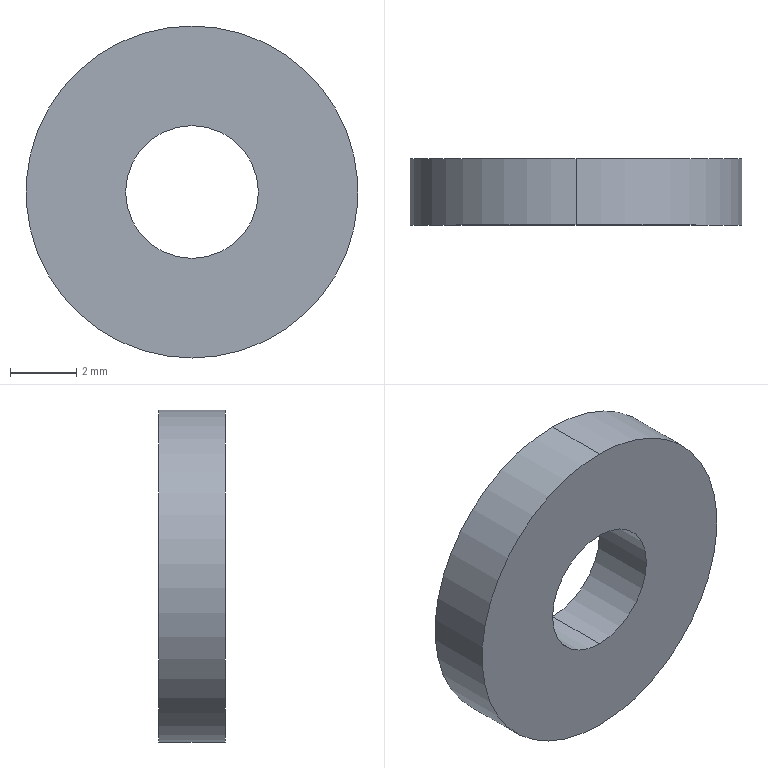Part | STEP file | Guide rail bracket shim 1001 | 1 solid | 6 faces | box 10 x 2 x 10 mm | volume 131.947 mm3 | cylinder 4 | plane 2 | commonest cylinder face diameters 4 x2 10 x2
STEP:
#1=CARTESIAN_POINT('',(0.,0.,0.));
#2=DIRECTION('',(0.,0.,1.));
#3=DIRECTION('',(1.,0.,0.));
#4=AXIS2_PLACEMENT_3D('',#1,#2,#3);
#5=CARTESIAN_POINT('',(0.,2.,-2.));
#6=VERTEX_POINT('',#5);
#7=CARTESIAN_POINT('',(0.,0.,-2.));
#8=VERTEX_POINT('',#7);
#9=CARTESIAN_POINT('',(0.,2.,-2.));
#10=DIRECTION('',(0.,-1.,0.));
#11=VECTOR('',#10,1.);
#12=LINE('',#9,#11);
#13=CARTESIAN_POINT('',(0.,2.,0.));
#14=DIRECTION('',(0.,-1.,0.));
#15=DIRECTION('',(0.,0.,-1.));
#16=AXIS2_PLACEMENT_3D('',#13,#14,#15);
#17=CYLINDRICAL_SURFACE('',#16,2.);
#18=CARTESIAN_POINT('',(6.283,0.));
#19=DIRECTION('',(0.,1.));
#20=VECTOR('',#19,1.);
#21=LINE('',#18,#20);
#22=(GEOMETRIC_REPRESENTATION_CONTEXT(2)PARAMETRIC_REPRESENTATION_CONTEXT()REPRESENTATION_CONTEXT('',''));
#23=DEFINITIONAL_REPRESENTATION('',(#21),#22);
#24=PCURVE('',#17,#23);
#25=CARTESIAN_POINT('',(0.,2.,0.));
#26=DIRECTION('',(0.,-1.,0.));
#27=DIRECTION('',(0.,0.,-1.));
#28=AXIS2_PLACEMENT_3D('',#25,#26,#27);
#29=CYLINDRICAL_SURFACE('',#28,2.);
#30=CARTESIAN_POINT('',(0.,0.));
#31=DIRECTION('',(0.,1.));
#32=VECTOR('',#31,1.);
#33=LINE('',#30,#32);
#34=(GEOMETRIC_REPRESENTATION_CONTEXT(2)PARAMETRIC_REPRESENTATION_CONTEXT()REPRESENTATION_CONTEXT('',''));
#35=DEFINITIONAL_REPRESENTATION('',(#33),#34);
#36=PCURVE('',#29,#35);
#37=SURFACE_CURVE('',#12,(#24,#36),.PCURVE_S1.);
#38=EDGE_CURVE('',#6,#8,#37,.T.);
#39=ORIENTED_EDGE('',*,*,#38,.T.);
#40=CARTESIAN_POINT('',(0.,0.,2.));
#41=VERTEX_POINT('',#40);
#42=CARTESIAN_POINT('',(0.,0.,0.));
#43=DIRECTION('',(0.,1.,0.));
#44=DIRECTION('',(0.,0.,1.));
#45=AXIS2_PLACEMENT_3D('',#42,#43,#44);
#46=CIRCLE('',#45,2.);
#47=CARTESIAN_POINT('',(9.425,2.));
#48=DIRECTION('',(-1.,0.));
#49=VECTOR('',#48,1.);
#50=LINE('',#47,#49);
#51=(GEOMETRIC_REPRESENTATION_CONTEXT(2)PARAMETRIC_REPRESENTATION_CONTEXT()REPRESENTATION_CONTEXT('',''));
#52=DEFINITIONAL_REPRESENTATION('',(#50),#51);
#53=PCURVE('',#17,#52);
#54=CARTESIAN_POINT('',(0.,0.,0.));
#55=DIRECTION('',(0.,1.,0.));
#56=DIRECTION('',(0.,0.,1.));
#57=AXIS2_PLACEMENT_3D('',#54,#55,#56);
#58=PLANE('',#57);
#59=CARTESIAN_POINT('',(0.,0.));
#60=DIRECTION('',(1.,0.));
#61=AXIS2_PLACEMENT_2D('',#59,#60);
#62=CIRCLE('',#61,2.);
#63=(GEOMETRIC_REPRESENTATION_CONTEXT(2)PARAMETRIC_REPRESENTATION_CONTEXT()REPRESENTATION_CONTEXT('',''));
#64=DEFINITIONAL_REPRESENTATION('',(#62),#63);
#65=PCURVE('',#58,#64);
#66=SURFACE_CURVE('',#46,(#53,#65),.PCURVE_S1.);
#67=EDGE_CURVE('',#8,#41,#66,.T.);
#68=ORIENTED_EDGE('',*,*,#67,.T.);
#69=CARTESIAN_POINT('',(0.,2.,2.));
#70=VERTEX_POINT('',#69);
#71=CARTESIAN_POINT('',(0.,2.,2.));
#72=DIRECTION('',(0.,-1.,0.));
#73=VECTOR('',#72,1.);
#74=LINE('',#71,#73);
#75=CARTESIAN_POINT('',(3.142,0.));
#76=DIRECTION('',(0.,1.));
#77=VECTOR('',#76,1.);
#78=LINE('',#75,#77);
#79=(GEOMETRIC_REPRESENTATION_CONTEXT(2)PARAMETRIC_REPRESENTATION_CONTEXT()REPRESENTATION_CONTEXT('',''));
#80=DEFINITIONAL_REPRESENTATION('',(#78),#79);
#81=PCURVE('',#17,#80);
#82=CARTESIAN_POINT('',(3.142,0.));
#83=DIRECTION('',(0.,1.));
#84=VECTOR('',#83,1.);
#85=LINE('',#82,#84);
#86=(GEOMETRIC_REPRESENTATION_CONTEXT(2)PARAMETRIC_REPRESENTATION_CONTEXT()REPRESENTATION_CONTEXT('',''));
#87=DEFINITIONAL_REPRESENTATION('',(#85),#86);
#88=PCURVE('',#29,#87);
#89=SURFACE_CURVE('',#74,(#81,#88),.PCURVE_S1.);
#90=EDGE_CURVE('',#70,#41,#89,.T.);
#91=ORIENTED_EDGE('',*,*,#90,.F.);
#92=CARTESIAN_POINT('',(0.,2.,0.));
#93=DIRECTION('',(0.,1.,0.));
#94=DIRECTION('',(0.,0.,1.));
#95=AXIS2_PLACEMENT_3D('',#92,#93,#94);
#96=CIRCLE('',#95,2.);
#97=CARTESIAN_POINT('',(9.425,0.));
#98=DIRECTION('',(-1.,0.));
#99=VECTOR('',#98,1.);
#100=LINE('',#97,#99);
#101=(GEOMETRIC_REPRESENTATION_CONTEXT(2)PARAMETRIC_REPRESENTATION_CONTEXT()REPRESENTATION_CONTEXT('',''));
#102=DEFINITIONAL_REPRESENTATION('',(#100),#101);
#103=PCURVE('',#17,#102);
#104=CARTESIAN_POINT('',(0.,2.,0.));
#105=DIRECTION('',(0.,1.,0.));
#106=DIRECTION('',(0.,0.,1.));
#107=AXIS2_PLACEMENT_3D('',#104,#105,#106);
#108=PLANE('',#107);
#109=CARTESIAN_POINT('',(0.,0.));
#110=DIRECTION('',(1.,0.));
#111=AXIS2_PLACEMENT_2D('',#109,#110);
#112=CIRCLE('',#111,2.);
#113=(GEOMETRIC_REPRESENTATION_CONTEXT(2)PARAMETRIC_REPRESENTATION_CONTEXT()REPRESENTATION_CONTEXT('',''));
#114=DEFINITIONAL_REPRESENTATION('',(#112),#113);
#115=PCURVE('',#108,#114);
#116=SURFACE_CURVE('',#96,(#103,#115),.PCURVE_S1.);
#117=EDGE_CURVE('',#6,#70,#116,.T.);
#118=ORIENTED_EDGE('',*,*,#117,.F.);
#119=EDGE_LOOP('',(#39,#68,#91,#118));
#120=FACE_BOUND('',#119,.F.);
#121=ADVANCED_FACE('',(#120),#17,.F.);
#122=CARTESIAN_POINT('',(0.,2.,5.));
#123=VERTEX_POINT('',#122);
#124=CARTESIAN_POINT('',(0.,2.,-5.));
#125=VERTEX_POINT('',#124);
#126=CARTESIAN_POINT('',(0.,2.,0.));
#127=DIRECTION('',(0.,1.,0.));
#128=DIRECTION('',(0.,0.,1.));
#129=AXIS2_PLACEMENT_3D('',#126,#127,#128);
#130=CIRCLE('',#129,5.);
#131=CARTESIAN_POINT('',(0.,2.,0.));
#132=DIRECTION('',(0.,-1.,0.));
#133=DIRECTION('',(0.,0.,-1.));
#134=AXIS2_PLACEMENT_3D('',#131,#132,#133);
#135=CYLINDRICAL_SURFACE('',#134,5.);
#136=CARTESIAN_POINT('',(3.142,0.));
#137=DIRECTION('',(-1.,0.));
#138=VECTOR('',#137,1.);
#139=LINE('',#136,#138);
#140=(GEOMETRIC_REPRESENTATION_CONTEXT(2)PARAMETRIC_REPRESENTATION_CONTEXT()REPRESENTATION_CONTEXT('',''));
#141=DEFINITIONAL_REPRESENTATION('',(#139),#140);
#142=PCURVE('',#135,#141);
#143=CARTESIAN_POINT('',(0.,0.));
#144=DIRECTION('',(1.,0.));
#145=AXIS2_PLACEMENT_2D('',#143,#144);
#146=CIRCLE('',#145,5.);
#147=(GEOMETRIC_REPRESENTATION_CONTEXT(2)PARAMETRIC_REPRESENTATION_CONTEXT()REPRESENTATION_CONTEXT('',''));
#148=DEFINITIONAL_REPRESENTATION('',(#146),#147);
#149=PCURVE('',#108,#148);
#150=SURFACE_CURVE('',#130,(#142,#149),.PCURVE_S1.);
#151=EDGE_CURVE('',#123,#125,#150,.T.);
#152=ORIENTED_EDGE('',*,*,#151,.F.);
#153=CARTESIAN_POINT('',(0.,0.,5.));
#154=VERTEX_POINT('',#153);
#155=CARTESIAN_POINT('',(0.,2.,5.));
#156=DIRECTION('',(0.,-1.,0.));
#157=VECTOR('',#156,1.);
#158=LINE('',#155,#157);
#159=CARTESIAN_POINT('',(3.142,0.));
#160=DIRECTION('',(0.,1.));
#161=VECTOR('',#160,1.);
#162=LINE('',#159,#161);
#163=(GEOMETRIC_REPRESENTATION_CONTEXT(2)PARAMETRIC_REPRESENTATION_CONTEXT()REPRESENTATION_CONTEXT('',''));
#164=DEFINITIONAL_REPRESENTATION('',(#162),#163);
#165=PCURVE('',#135,#164);
#166=CARTESIAN_POINT('',(0.,2.,0.));
#167=DIRECTION('',(0.,-1.,0.));
#168=DIRECTION('',(0.,0.,-1.));
#169=AXIS2_PLACEMENT_3D('',#166,#167,#168);
#170=CYLINDRICAL_SURFACE('',#169,5.);
#171=CARTESIAN_POINT('',(3.142,0.));
#172=DIRECTION('',(0.,1.));
#173=VECTOR('',#172,1.);
#174=LINE('',#171,#173);
#175=(GEOMETRIC_REPRESENTATION_CONTEXT(2)PARAMETRIC_REPRESENTATION_CONTEXT()REPRESENTATION_CONTEXT('',''));
#176=DEFINITIONAL_REPRESENTATION('',(#174),#175);
#177=PCURVE('',#170,#176);
#178=SURFACE_CURVE('',#158,(#165,#177),.PCURVE_S1.);
#179=EDGE_CURVE('',#123,#154,#178,.T.);
#180=ORIENTED_EDGE('',*,*,#179,.T.);
#181=CARTESIAN_POINT('',(0.,0.,-5.));
#182=VERTEX_POINT('',#181);
#183=CARTESIAN_POINT('',(0.,0.,0.));
#184=DIRECTION('',(0.,1.,0.));
#185=DIRECTION('',(0.,0.,1.));
#186=AXIS2_PLACEMENT_3D('',#183,#184,#185);
#187=CIRCLE('',#186,5.);
#188=CARTESIAN_POINT('',(3.142,2.));
#189=DIRECTION('',(-1.,0.));
#190=VECTOR('',#189,1.);
#191=LINE('',#188,#190);
#192=(GEOMETRIC_REPRESENTATION_CONTEXT(2)PARAMETRIC_REPRESENTATION_CONTEXT()REPRESENTATION_CONTEXT('',''));
#193=DEFINITIONAL_REPRESENTATION('',(#191),#192);
#194=PCURVE('',#135,#193);
#195=CARTESIAN_POINT('',(0.,0.));
#196=DIRECTION('',(1.,0.));
#197=AXIS2_PLACEMENT_2D('',#195,#196);
#198=CIRCLE('',#197,5.);
#199=(GEOMETRIC_REPRESENTATION_CONTEXT(2)PARAMETRIC_REPRESENTATION_CONTEXT()REPRESENTATION_CONTEXT('',''));
#200=DEFINITIONAL_REPRESENTATION('',(#198),#199);
#201=PCURVE('',#58,#200);
#202=SURFACE_CURVE('',#187,(#194,#201),.PCURVE_S1.);
#203=EDGE_CURVE('',#154,#182,#202,.T.);
#204=ORIENTED_EDGE('',*,*,#203,.T.);
#205=CARTESIAN_POINT('',(0.,2.,-5.));
#206=DIRECTION('',(0.,-1.,0.));
#207=VECTOR('',#206,1.);
#208=LINE('',#205,#207);
#209=CARTESIAN_POINT('',(0.,0.));
#210=DIRECTION('',(0.,1.));
#211=VECTOR('',#210,1.);
#212=LINE('',#209,#211);
#213=(GEOMETRIC_REPRESENTATION_CONTEXT(2)PARAMETRIC_REPRESENTATION_CONTEXT()REPRESENTATION_CONTEXT('',''));
#214=DEFINITIONAL_REPRESENTATION('',(#212),#213);
#215=PCURVE('',#135,#214);
#216=CARTESIAN_POINT('',(6.283,0.));
#217=DIRECTION('',(0.,1.));
#218=VECTOR('',#217,1.);
#219=LINE('',#216,#218);
#220=(GEOMETRIC_REPRESENTATION_CONTEXT(2)PARAMETRIC_REPRESENTATION_CONTEXT()REPRESENTATION_CONTEXT('',''));
#221=DEFINITIONAL_REPRESENTATION('',(#219),#220);
#222=PCURVE('',#170,#221);
#223=SURFACE_CURVE('',#208,(#215,#222),.PCURVE_S1.);
#224=EDGE_CURVE('',#125,#182,#223,.T.);
#225=ORIENTED_EDGE('',*,*,#224,.F.);
#226=EDGE_LOOP('',(#152,#180,#204,#225));
#227=FACE_BOUND('',#226,.T.);
#228=ADVANCED_FACE('',(#227),#135,.T.);
#229=CARTESIAN_POINT('',(0.,2.,0.));
#230=DIRECTION('',(0.,1.,0.));
#231=DIRECTION('',(0.,0.,1.));
#232=AXIS2_PLACEMENT_3D('',#229,#230,#231);
#233=CIRCLE('',#232,5.);
#234=CARTESIAN_POINT('',(0.,0.));
#235=DIRECTION('',(1.,0.));
#236=AXIS2_PLACEMENT_2D('',#234,#235);
#237=CIRCLE('',#236,5.);
#238=(GEOMETRIC_REPRESENTATION_CONTEXT(2)PARAMETRIC_REPRESENTATION_CONTEXT()REPRESENTATION_CONTEXT('',''));
#239=DEFINITIONAL_REPRESENTATION('',(#237),#238);
#240=PCURVE('',#108,#239);
#241=CARTESIAN_POINT('',(9.425,0.));
#242=DIRECTION('',(-1.,0.));
#243=VECTOR('',#242,1.);
#244=LINE('',#241,#243);
#245=(GEOMETRIC_REPRESENTATION_CONTEXT(2)PARAMETRIC_REPRESENTATION_CONTEXT()REPRESENTATION_CONTEXT('',''));
#246=DEFINITIONAL_REPRESENTATION('',(#244),#245);
#247=PCURVE('',#170,#246);
#248=SURFACE_CURVE('',#233,(#240,#247),.PCURVE_S1.);
#249=EDGE_CURVE('',#125,#123,#248,.T.);
#250=ORIENTED_EDGE('',*,*,#249,.T.);
#251=ORIENTED_EDGE('',*,*,#151,.T.);
#252=EDGE_LOOP('',(#250,#251));
#253=FACE_BOUND('',#252,.T.);
#254=ORIENTED_EDGE('',*,*,#117,.F.);
#255=CARTESIAN_POINT('',(0.,2.,0.));
#256=DIRECTION('',(0.,1.,0.));
#257=DIRECTION('',(0.,0.,1.));
#258=AXIS2_PLACEMENT_3D('',#255,#256,#257);
#259=CIRCLE('',#258,2.);
#260=CARTESIAN_POINT('',(0.,0.));
#261=DIRECTION('',(1.,0.));
#262=AXIS2_PLACEMENT_2D('',#260,#261);
#263=CIRCLE('',#262,2.);
#264=(GEOMETRIC_REPRESENTATION_CONTEXT(2)PARAMETRIC_REPRESENTATION_CONTEXT()REPRESENTATION_CONTEXT('',''));
#265=DEFINITIONAL_REPRESENTATION('',(#263),#264);
#266=PCURVE('',#108,#265);
#267=CARTESIAN_POINT('',(3.142,0.));
#268=DIRECTION('',(-1.,0.));
#269=VECTOR('',#268,1.);
#270=LINE('',#267,#269);
#271=(GEOMETRIC_REPRESENTATION_CONTEXT(2)PARAMETRIC_REPRESENTATION_CONTEXT()REPRESENTATION_CONTEXT('',''));
#272=DEFINITIONAL_REPRESENTATION('',(#270),#271);
#273=PCURVE('',#29,#272);
#274=SURFACE_CURVE('',#259,(#266,#273),.PCURVE_S1.);
#275=EDGE_CURVE('',#70,#6,#274,.T.);
#276=ORIENTED_EDGE('',*,*,#275,.F.);
#277=EDGE_LOOP('',(#254,#276));
#278=FACE_BOUND('',#277,.T.);
#279=ADVANCED_FACE('',(#253,#278),#108,.T.);
#280=CARTESIAN_POINT('',(0.,0.,0.));
#281=DIRECTION('',(0.,1.,0.));
#282=DIRECTION('',(0.,0.,1.));
#283=AXIS2_PLACEMENT_3D('',#280,#281,#282);
#284=CIRCLE('',#283,5.);
#285=CARTESIAN_POINT('',(0.,0.));
#286=DIRECTION('',(1.,0.));
#287=AXIS2_PLACEMENT_2D('',#285,#286);
#288=CIRCLE('',#287,5.);
#289=(GEOMETRIC_REPRESENTATION_CONTEXT(2)PARAMETRIC_REPRESENTATION_CONTEXT()REPRESENTATION_CONTEXT('',''));
#290=DEFINITIONAL_REPRESENTATION('',(#288),#289);
#291=PCURVE('',#58,#290);
#292=CARTESIAN_POINT('',(9.425,2.));
#293=DIRECTION('',(-1.,0.));
#294=VECTOR('',#293,1.);
#295=LINE('',#292,#294);
#296=(GEOMETRIC_REPRESENTATION_CONTEXT(2)PARAMETRIC_REPRESENTATION_CONTEXT()REPRESENTATION_CONTEXT('',''));
#297=DEFINITIONAL_REPRESENTATION('',(#295),#296);
#298=PCURVE('',#170,#297);
#299=SURFACE_CURVE('',#284,(#291,#298),.PCURVE_S1.);
#300=EDGE_CURVE('',#182,#154,#299,.T.);
#301=ORIENTED_EDGE('',*,*,#300,.F.);
#302=ORIENTED_EDGE('',*,*,#203,.F.);
#303=EDGE_LOOP('',(#301,#302));
#304=FACE_BOUND('',#303,.T.);
#305=ORIENTED_EDGE('',*,*,#67,.T.);
#306=CARTESIAN_POINT('',(0.,0.,0.));
#307=DIRECTION('',(0.,1.,0.));
#308=DIRECTION('',(0.,0.,1.));
#309=AXIS2_PLACEMENT_3D('',#306,#307,#308);
#310=CIRCLE('',#309,2.);
#311=CARTESIAN_POINT('',(0.,0.));
#312=DIRECTION('',(1.,0.));
#313=AXIS2_PLACEMENT_2D('',#311,#312);
#314=CIRCLE('',#313,2.);
#315=(GEOMETRIC_REPRESENTATION_CONTEXT(2)PARAMETRIC_REPRESENTATION_CONTEXT()REPRESENTATION_CONTEXT('',''));
#316=DEFINITIONAL_REPRESENTATION('',(#314),#315);
#317=PCURVE('',#58,#316);
#318=CARTESIAN_POINT('',(3.142,2.));
#319=DIRECTION('',(-1.,0.));
#320=VECTOR('',#319,1.);
#321=LINE('',#318,#320);
#322=(GEOMETRIC_REPRESENTATION_CONTEXT(2)PARAMETRIC_REPRESENTATION_CONTEXT()REPRESENTATION_CONTEXT('',''));
#323=DEFINITIONAL_REPRESENTATION('',(#321),#322);
#324=PCURVE('',#29,#323);
#325=SURFACE_CURVE('',#310,(#317,#324),.PCURVE_S1.);
#326=EDGE_CURVE('',#41,#8,#325,.T.);
#327=ORIENTED_EDGE('',*,*,#326,.T.);
#328=EDGE_LOOP('',(#305,#327));
#329=FACE_BOUND('',#328,.T.);
#330=ADVANCED_FACE('',(#304,#329),#58,.F.);
#331=ORIENTED_EDGE('',*,*,#179,.F.);
#332=ORIENTED_EDGE('',*,*,#249,.F.);
#333=ORIENTED_EDGE('',*,*,#224,.T.);
#334=ORIENTED_EDGE('',*,*,#300,.T.);
#335=EDGE_LOOP('',(#331,#332,#333,#334));
#336=FACE_BOUND('',#335,.T.);
#337=ADVANCED_FACE('',(#336),#170,.T.);
#338=ORIENTED_EDGE('',*,*,#326,.T.);
#339=ORIENTED_EDGE('',*,*,#38,.F.);
#340=ORIENTED_EDGE('',*,*,#275,.F.);
#341=ORIENTED_EDGE('',*,*,#90,.T.);
#342=EDGE_LOOP('',(#338,#339,#340,#341));
#343=FACE_BOUND('',#342,.F.);
#344=ADVANCED_FACE('',(#343),#29,.F.);
#345=CLOSED_SHELL('',(#121,#228,#279,#330,#337,#344));
#346=MANIFOLD_SOLID_BREP('',#345);
#347=(LENGTH_UNIT()NAMED_UNIT(*)SI_UNIT(.MILLI.,.METRE.));
#348=UNCERTAINTY_MEASURE_WITH_UNIT(LENGTH_MEASURE(0.0000001),#347,'','');
#349=(NAMED_UNIT(*)PLANE_ANGLE_UNIT()SI_UNIT($,.RADIAN.));
#350=(NAMED_UNIT(*)SI_UNIT($,.STERADIAN.)SOLID_ANGLE_UNIT());
#351=(GEOMETRIC_REPRESENTATION_CONTEXT(3)GLOBAL_UNCERTAINTY_ASSIGNED_CONTEXT((#348))GLOBAL_UNIT_ASSIGNED_CONTEXT((#347,#349,#350))REPRESENTATION_CONTEXT('',''));
#352=ADVANCED_BREP_SHAPE_REPRESENTATION('',(#4,#346),#351);